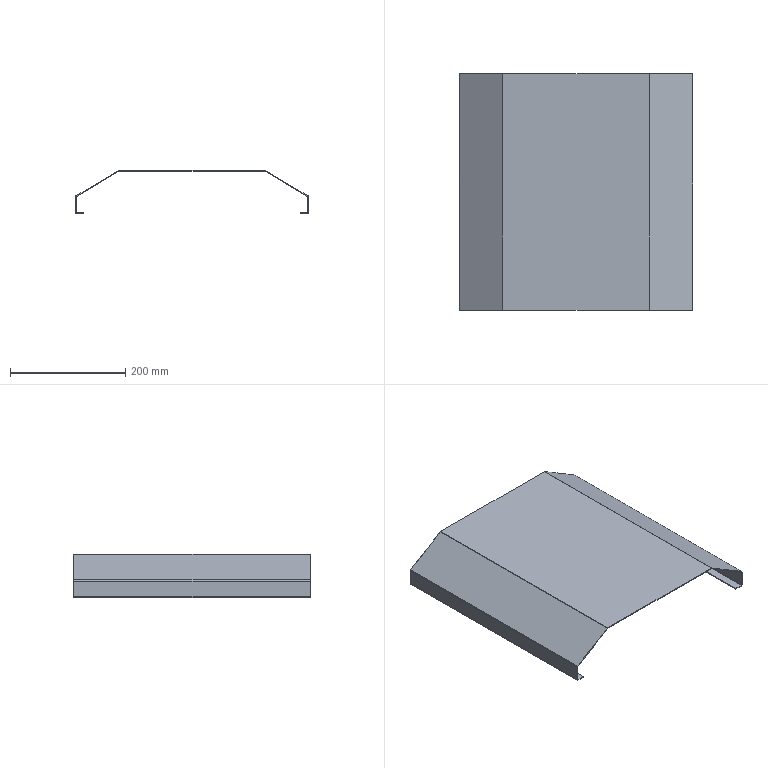Part | SolidWorks | features BaseBody 1 | 1 solid | 38 faces | box 405 x 410 x 75 mm | volume 315141 mm3 | cylinder 20 | plane 18 | commonest cylinder face diameters 6.8 x8 1.473 x6 4.473 x6
STEP:
#1=CARTESIAN_POINT('',(201.,65.5,-54.6));
#2=VERTEX_POINT('',#1);
#3=CARTESIAN_POINT('',(201.,65.5,-61.4));
#4=VERTEX_POINT('',#3);
#5=CARTESIAN_POINT('',(201.,65.5,-58.));
#6=DIRECTION('',(1.,0.,0.));
#7=DIRECTION('',(0.,0.,-1.));
#8=AXIS2_PLACEMENT_3D('',#5,#6,#7);
#9=CIRCLE('',#8,3.4);
#10=EDGE_CURVE('',#2,#4,#9,.T.);
#11=ORIENTED_EDGE('',*,*,#10,.F.);
#12=CARTESIAN_POINT('',(202.5,65.5,-54.6));
#13=VERTEX_POINT('',#12);
#14=CARTESIAN_POINT('',(202.5,65.5,-54.6));
#15=DIRECTION('',(1.,0.,0.));
#16=VECTOR('',#15,1000.);
#17=LINE('',#14,#16);
#18=EDGE_CURVE('',#2,#13,#17,.T.);
#19=ORIENTED_EDGE('',*,*,#18,.T.);
#20=CARTESIAN_POINT('',(202.5,65.5,-61.4));
#21=VERTEX_POINT('',#20);
#22=CARTESIAN_POINT('',(202.5,65.5,-58.));
#23=DIRECTION('',(-1.,0.,0.));
#24=DIRECTION('',(0.,0.,-1.));
#25=AXIS2_PLACEMENT_3D('',#22,#23,#24);
#26=CIRCLE('',#25,3.4);
#27=EDGE_CURVE('',#21,#13,#26,.T.);
#28=ORIENTED_EDGE('',*,*,#27,.F.);
#29=CARTESIAN_POINT('',(202.5,65.5,-61.4));
#30=DIRECTION('',(1.,0.,0.));
#31=VECTOR('',#30,1000.);
#32=LINE('',#29,#31);
#33=EDGE_CURVE('',#4,#21,#32,.T.);
#34=ORIENTED_EDGE('',*,*,#33,.F.);
#35=EDGE_LOOP('',(#11,#19,#28,#34));
#36=FACE_OUTER_BOUND('',#35,.T.);
#37=CARTESIAN_POINT('',(202.5,65.5,-58.));
#38=DIRECTION('',(1.,0.,0.));
#39=DIRECTION('',(0.,0.,-1.));
#40=AXIS2_PLACEMENT_3D('',#37,#38,#39);
#41=CYLINDRICAL_SURFACE('',#40,3.4);
#42=ADVANCED_FACE('',(#36),#41,.F.);
#43=CARTESIAN_POINT('',(201.,101.5,-54.6));
#44=VERTEX_POINT('',#43);
#45=CARTESIAN_POINT('',(201.,101.5,-61.4));
#46=VERTEX_POINT('',#45);
#47=CARTESIAN_POINT('',(201.,101.5,-58.));
#48=DIRECTION('',(1.,0.,0.));
#49=DIRECTION('',(0.,0.,-1.));
#50=AXIS2_PLACEMENT_3D('',#47,#48,#49);
#51=CIRCLE('',#50,3.4);
#52=EDGE_CURVE('',#44,#46,#51,.T.);
#53=ORIENTED_EDGE('',*,*,#52,.F.);
#54=CARTESIAN_POINT('',(202.5,101.5,-54.6));
#55=VERTEX_POINT('',#54);
#56=CARTESIAN_POINT('',(202.5,101.5,-54.6));
#57=DIRECTION('',(1.,0.,0.));
#58=VECTOR('',#57,1000.);
#59=LINE('',#56,#58);
#60=EDGE_CURVE('',#44,#55,#59,.T.);
#61=ORIENTED_EDGE('',*,*,#60,.T.);
#62=CARTESIAN_POINT('',(202.5,101.5,-61.4));
#63=VERTEX_POINT('',#62);
#64=CARTESIAN_POINT('',(202.5,101.5,-58.));
#65=DIRECTION('',(-1.,0.,0.));
#66=DIRECTION('',(0.,0.,-1.));
#67=AXIS2_PLACEMENT_3D('',#64,#65,#66);
#68=CIRCLE('',#67,3.4);
#69=EDGE_CURVE('',#63,#55,#68,.T.);
#70=ORIENTED_EDGE('',*,*,#69,.F.);
#71=CARTESIAN_POINT('',(202.5,101.5,-61.4));
#72=DIRECTION('',(1.,0.,0.));
#73=VECTOR('',#72,1000.);
#74=LINE('',#71,#73);
#75=EDGE_CURVE('',#46,#63,#74,.T.);
#76=ORIENTED_EDGE('',*,*,#75,.F.);
#77=EDGE_LOOP('',(#53,#61,#70,#76));
#78=FACE_OUTER_BOUND('',#77,.T.);
#79=CARTESIAN_POINT('',(202.5,101.5,-58.));
#80=DIRECTION('',(1.,0.,0.));
#81=DIRECTION('',(0.,0.,-1.));
#82=AXIS2_PLACEMENT_3D('',#79,#80,#81);
#83=CYLINDRICAL_SURFACE('',#82,3.4);
#84=ADVANCED_FACE('',(#78),#83,.F.);
#85=CARTESIAN_POINT('',(201.,241.5,-54.6));
#86=VERTEX_POINT('',#85);
#87=CARTESIAN_POINT('',(201.,241.5,-61.4));
#88=VERTEX_POINT('',#87);
#89=CARTESIAN_POINT('',(201.,241.5,-58.));
#90=DIRECTION('',(1.,0.,0.));
#91=DIRECTION('',(0.,0.,-1.));
#92=AXIS2_PLACEMENT_3D('',#89,#90,#91);
#93=CIRCLE('',#92,3.4);
#94=EDGE_CURVE('',#86,#88,#93,.T.);
#95=ORIENTED_EDGE('',*,*,#94,.F.);
#96=CARTESIAN_POINT('',(202.5,241.5,-54.6));
#97=VERTEX_POINT('',#96);
#98=CARTESIAN_POINT('',(202.5,241.5,-54.6));
#99=DIRECTION('',(1.,0.,0.));
#100=VECTOR('',#99,1000.);
#101=LINE('',#98,#100);
#102=EDGE_CURVE('',#86,#97,#101,.T.);
#103=ORIENTED_EDGE('',*,*,#102,.T.);
#104=CARTESIAN_POINT('',(202.5,241.5,-61.4));
#105=VERTEX_POINT('',#104);
#106=CARTESIAN_POINT('',(202.5,241.5,-58.));
#107=DIRECTION('',(-1.,0.,0.));
#108=DIRECTION('',(0.,0.,-1.));
#109=AXIS2_PLACEMENT_3D('',#106,#107,#108);
#110=CIRCLE('',#109,3.4);
#111=EDGE_CURVE('',#105,#97,#110,.T.);
#112=ORIENTED_EDGE('',*,*,#111,.F.);
#113=CARTESIAN_POINT('',(202.5,241.5,-61.4));
#114=DIRECTION('',(1.,0.,0.));
#115=VECTOR('',#114,1000.);
#116=LINE('',#113,#115);
#117=EDGE_CURVE('',#88,#105,#116,.T.);
#118=ORIENTED_EDGE('',*,*,#117,.F.);
#119=EDGE_LOOP('',(#95,#103,#112,#118));
#120=FACE_OUTER_BOUND('',#119,.T.);
#121=CARTESIAN_POINT('',(202.5,241.5,-58.));
#122=DIRECTION('',(1.,0.,0.));
#123=DIRECTION('',(0.,0.,-1.));
#124=AXIS2_PLACEMENT_3D('',#121,#122,#123);
#125=CYLINDRICAL_SURFACE('',#124,3.4);
#126=ADVANCED_FACE('',(#120),#125,.F.);
#127=CARTESIAN_POINT('',(201.,277.5,-54.6));
#128=VERTEX_POINT('',#127);
#129=CARTESIAN_POINT('',(201.,277.5,-61.4));
#130=VERTEX_POINT('',#129);
#131=CARTESIAN_POINT('',(201.,277.5,-58.));
#132=DIRECTION('',(1.,0.,0.));
#133=DIRECTION('',(0.,0.,-1.));
#134=AXIS2_PLACEMENT_3D('',#131,#132,#133);
#135=CIRCLE('',#134,3.4);
#136=EDGE_CURVE('',#128,#130,#135,.T.);
#137=ORIENTED_EDGE('',*,*,#136,.F.);
#138=CARTESIAN_POINT('',(202.5,277.5,-54.6));
#139=VERTEX_POINT('',#138);
#140=CARTESIAN_POINT('',(202.5,277.5,-54.6));
#141=DIRECTION('',(1.,0.,0.));
#142=VECTOR('',#141,1000.);
#143=LINE('',#140,#142);
#144=EDGE_CURVE('',#128,#139,#143,.T.);
#145=ORIENTED_EDGE('',*,*,#144,.T.);
#146=CARTESIAN_POINT('',(202.5,277.5,-61.4));
#147=VERTEX_POINT('',#146);
#148=CARTESIAN_POINT('',(202.5,277.5,-58.));
#149=DIRECTION('',(-1.,0.,0.));
#150=DIRECTION('',(0.,0.,-1.));
#151=AXIS2_PLACEMENT_3D('',#148,#149,#150);
#152=CIRCLE('',#151,3.4);
#153=EDGE_CURVE('',#147,#139,#152,.T.);
#154=ORIENTED_EDGE('',*,*,#153,.F.);
#155=CARTESIAN_POINT('',(202.5,277.5,-61.4));
#156=DIRECTION('',(1.,0.,0.));
#157=VECTOR('',#156,1000.);
#158=LINE('',#155,#157);
#159=EDGE_CURVE('',#130,#147,#158,.T.);
#160=ORIENTED_EDGE('',*,*,#159,.F.);
#161=EDGE_LOOP('',(#137,#145,#154,#160));
#162=FACE_OUTER_BOUND('',#161,.T.);
#163=CARTESIAN_POINT('',(202.5,277.5,-58.));
#164=DIRECTION('',(1.,0.,0.));
#165=DIRECTION('',(0.,0.,-1.));
#166=AXIS2_PLACEMENT_3D('',#163,#164,#165);
#167=CYLINDRICAL_SURFACE('',#166,3.4);
#168=ADVANCED_FACE('',(#162),#167,.F.);
#169=CARTESIAN_POINT('',(-126.88,410.,-1.5));
#170=VERTEX_POINT('',#169);
#171=CARTESIAN_POINT('',(126.88,410.,-1.5));
#172=VERTEX_POINT('',#171);
#173=CARTESIAN_POINT('',(-127.5,410.,-1.5));
#174=DIRECTION('',(1.,0.,0.));
#175=VECTOR('',#174,1000.);
#176=LINE('',#173,#175);
#177=EDGE_CURVE('',#170,#172,#176,.T.);
#178=ORIENTED_EDGE('',*,*,#177,.T.);
#179=CARTESIAN_POINT('',(126.88,0.,-1.5));
#180=VERTEX_POINT('',#179);
#181=CARTESIAN_POINT('',(126.88,410.,-1.5));
#182=DIRECTION('',(0.,-1.,0.));
#183=VECTOR('',#182,1000.);
#184=LINE('',#181,#183);
#185=EDGE_CURVE('',#172,#180,#184,.T.);
#186=ORIENTED_EDGE('',*,*,#185,.T.);
#187=CARTESIAN_POINT('',(-126.88,0.,-1.5));
#188=VERTEX_POINT('',#187);
#189=CARTESIAN_POINT('',(-127.5,0.,-1.5));
#190=DIRECTION('',(-1.,0.,0.));
#191=VECTOR('',#190,1000.);
#192=LINE('',#189,#191);
#193=EDGE_CURVE('',#180,#188,#192,.T.);
#194=ORIENTED_EDGE('',*,*,#193,.T.);
#195=CARTESIAN_POINT('',(-126.88,410.,-1.5));
#196=DIRECTION('',(0.,1.,0.));
#197=VECTOR('',#196,1000.);
#198=LINE('',#195,#197);
#199=EDGE_CURVE('',#188,#170,#198,.T.);
#200=ORIENTED_EDGE('',*,*,#199,.T.);
#201=EDGE_LOOP('',(#178,#186,#194,#200));
#202=FACE_OUTER_BOUND('',#201,.T.);
#203=CARTESIAN_POINT('',(-127.5,410.,-1.5));
#204=DIRECTION('',(0.,0.,-1.));
#205=DIRECTION('',(-1.,0.,0.));
#206=AXIS2_PLACEMENT_3D('',#203,#204,#205);
#207=PLANE('',#206);
#208=ADVANCED_FACE('',(#202),#207,.T.);
#209=ORIENTED_EDGE('',*,*,#185,.F.);
#210=CARTESIAN_POINT('',(127.259,410.,-1.605));
#211=VERTEX_POINT('',#210);
#212=CARTESIAN_POINT('',(126.88,410.,-2.237));
#213=DIRECTION('',(0.,-1.,0.));
#214=DIRECTION('',(0.,0.,-1.));
#215=AXIS2_PLACEMENT_3D('',#212,#213,#214);
#216=CIRCLE('',#215,0.7366);
#217=EDGE_CURVE('',#211,#172,#216,.T.);
#218=ORIENTED_EDGE('',*,*,#217,.F.);
#219=CARTESIAN_POINT('',(127.259,0.,-1.605));
#220=VERTEX_POINT('',#219);
#221=CARTESIAN_POINT('',(127.259,410.,-1.605));
#222=DIRECTION('',(0.,1.,0.));
#223=VECTOR('',#222,1000.);
#224=LINE('',#221,#223);
#225=EDGE_CURVE('',#220,#211,#224,.T.);
#226=ORIENTED_EDGE('',*,*,#225,.F.);
#227=CARTESIAN_POINT('',(126.88,0.,-2.237));
#228=DIRECTION('',(0.,1.,0.));
#229=DIRECTION('',(0.,0.,-1.));
#230=AXIS2_PLACEMENT_3D('',#227,#228,#229);
#231=CIRCLE('',#230,0.7366);
#232=EDGE_CURVE('',#180,#220,#231,.T.);
#233=ORIENTED_EDGE('',*,*,#232,.F.);
#234=EDGE_LOOP('',(#209,#218,#226,#233));
#235=FACE_OUTER_BOUND('',#234,.T.);
#236=CARTESIAN_POINT('',(126.88,410.,-2.237));
#237=DIRECTION('',(0.,-1.,0.));
#238=DIRECTION('',(0.,0.,-1.));
#239=AXIS2_PLACEMENT_3D('',#236,#237,#238);
#240=CYLINDRICAL_SURFACE('',#239,0.7366);
#241=ADVANCED_FACE('',(#235),#240,.F.);
#242=ORIENTED_EDGE('',*,*,#177,.F.);
#243=CARTESIAN_POINT('',(-127.259,410.,-1.605));
#244=VERTEX_POINT('',#243);
#245=CARTESIAN_POINT('',(-126.88,410.,-2.237));
#246=DIRECTION('',(0.,-1.,0.));
#247=DIRECTION('',(0.,0.,-1.));
#248=AXIS2_PLACEMENT_3D('',#245,#246,#247);
#249=CIRCLE('',#248,0.7366);
#250=EDGE_CURVE('',#170,#244,#249,.T.);
#251=ORIENTED_EDGE('',*,*,#250,.T.);
#252=CARTESIAN_POINT('',(-200.642,410.,-45.635));
#253=VERTEX_POINT('',#252);
#254=CARTESIAN_POINT('',(-126.728,410.,-1.286));
#255=DIRECTION('',(0.8575,0.,0.5145));
#256=VECTOR('',#255,1000.);
#257=LINE('',#254,#256);
#258=EDGE_CURVE('',#253,#244,#257,.T.);
#259=ORIENTED_EDGE('',*,*,#258,.F.);
#260=CARTESIAN_POINT('',(-201.,410.,-46.266));
#261=VERTEX_POINT('',#260);
#262=CARTESIAN_POINT('',(-200.263,410.,-46.266));
#263=DIRECTION('',(0.,-1.,0.));
#264=DIRECTION('',(0.,0.,-1.));
#265=AXIS2_PLACEMENT_3D('',#262,#263,#264);
#266=CIRCLE('',#265,0.7366);
#267=EDGE_CURVE('',#253,#261,#266,.T.);
#268=ORIENTED_EDGE('',*,*,#267,.T.);
#269=CARTESIAN_POINT('',(-201.,410.,-72.763));
#270=VERTEX_POINT('',#269);
#271=CARTESIAN_POINT('',(-201.,410.,-45.));
#272=DIRECTION('',(0.,0.,1.));
#273=VECTOR('',#272,1000.);
#274=LINE('',#271,#273);
#275=EDGE_CURVE('',#270,#261,#274,.T.);
#276=ORIENTED_EDGE('',*,*,#275,.F.);
#277=CARTESIAN_POINT('',(-200.263,410.,-73.5));
#278=VERTEX_POINT('',#277);
#279=CARTESIAN_POINT('',(-200.263,410.,-72.763));
#280=DIRECTION('',(0.,-1.,0.));
#281=DIRECTION('',(0.,0.,-1.));
#282=AXIS2_PLACEMENT_3D('',#279,#280,#281);
#283=CIRCLE('',#282,0.7366);
#284=EDGE_CURVE('',#270,#278,#283,.T.);
#285=ORIENTED_EDGE('',*,*,#284,.T.);
#286=CARTESIAN_POINT('',(-187.5,410.,-73.5));
#287=VERTEX_POINT('',#286);
#288=CARTESIAN_POINT('',(-202.5,410.,-73.5));
#289=DIRECTION('',(-1.,0.,0.));
#290=VECTOR('',#289,1000.);
#291=LINE('',#288,#290);
#292=EDGE_CURVE('',#287,#278,#291,.T.);
#293=ORIENTED_EDGE('',*,*,#292,.F.);
#294=CARTESIAN_POINT('',(-187.5,410.,-75.));
#295=VERTEX_POINT('',#294);
#296=CARTESIAN_POINT('',(-187.5,410.,-72.763));
#297=DIRECTION('',(0.,0.,-1.));
#298=VECTOR('',#297,1000.);
#299=LINE('',#296,#298);
#300=EDGE_CURVE('',#287,#295,#299,.T.);
#301=ORIENTED_EDGE('',*,*,#300,.T.);
#302=CARTESIAN_POINT('',(-200.263,410.,-75.));
#303=VERTEX_POINT('',#302);
#304=CARTESIAN_POINT('',(-201.,410.,-75.));
#305=DIRECTION('',(-1.,0.,0.));
#306=VECTOR('',#305,1000.);
#307=LINE('',#304,#306);
#308=EDGE_CURVE('',#295,#303,#307,.T.);
#309=ORIENTED_EDGE('',*,*,#308,.T.);
#310=CARTESIAN_POINT('',(-202.5,410.,-72.763));
#311=VERTEX_POINT('',#310);
#312=CARTESIAN_POINT('',(-200.263,410.,-72.763));
#313=DIRECTION('',(0.,-1.,0.));
#314=DIRECTION('',(0.,0.,-1.));
#315=AXIS2_PLACEMENT_3D('',#312,#313,#314);
#316=CIRCLE('',#315,2.237);
#317=EDGE_CURVE('',#311,#303,#316,.T.);
#318=ORIENTED_EDGE('',*,*,#317,.F.);
#319=CARTESIAN_POINT('',(-202.5,410.,-46.266));
#320=VERTEX_POINT('',#319);
#321=CARTESIAN_POINT('',(-202.5,410.,-45.635));
#322=DIRECTION('',(0.,0.,1.));
#323=VECTOR('',#322,1000.);
#324=LINE('',#321,#323);
#325=EDGE_CURVE('',#311,#320,#324,.T.);
#326=ORIENTED_EDGE('',*,*,#325,.T.);
#327=CARTESIAN_POINT('',(-201.414,410.,-44.348));
#328=VERTEX_POINT('',#327);
#329=CARTESIAN_POINT('',(-200.263,410.,-46.266));
#330=DIRECTION('',(0.,-1.,0.));
#331=DIRECTION('',(0.,0.,-1.));
#332=AXIS2_PLACEMENT_3D('',#329,#330,#331);
#333=CIRCLE('',#332,2.237);
#334=EDGE_CURVE('',#328,#320,#333,.T.);
#335=ORIENTED_EDGE('',*,*,#334,.F.);
#336=CARTESIAN_POINT('',(-128.031,410.,-0.3187));
#337=VERTEX_POINT('',#336);
#338=CARTESIAN_POINT('',(-201.414,410.,-44.348));
#339=DIRECTION('',(0.8575,0.,0.5145));
#340=VECTOR('',#339,1000.);
#341=LINE('',#338,#340);
#342=EDGE_CURVE('',#328,#337,#341,.T.);
#343=ORIENTED_EDGE('',*,*,#342,.T.);
#344=CARTESIAN_POINT('',(-126.88,410.,0.));
#345=VERTEX_POINT('',#344);
#346=CARTESIAN_POINT('',(-126.88,410.,-2.237));
#347=DIRECTION('',(0.,-1.,0.));
#348=DIRECTION('',(0.,0.,-1.));
#349=AXIS2_PLACEMENT_3D('',#346,#347,#348);
#350=CIRCLE('',#349,2.237);
#351=EDGE_CURVE('',#345,#337,#350,.T.);
#352=ORIENTED_EDGE('',*,*,#351,.F.);
#353=CARTESIAN_POINT('',(126.88,410.,0.));
#354=VERTEX_POINT('',#353);
#355=CARTESIAN_POINT('',(127.259,410.,0.));
#356=DIRECTION('',(1.,0.,0.));
#357=VECTOR('',#356,1000.);
#358=LINE('',#355,#357);
#359=EDGE_CURVE('',#345,#354,#358,.T.);
#360=ORIENTED_EDGE('',*,*,#359,.T.);
#361=CARTESIAN_POINT('',(128.031,410.,-0.3187));
#362=VERTEX_POINT('',#361);
#363=CARTESIAN_POINT('',(126.88,410.,-2.237));
#364=DIRECTION('',(0.,-1.,0.));
#365=DIRECTION('',(0.,0.,-1.));
#366=AXIS2_PLACEMENT_3D('',#363,#364,#365);
#367=CIRCLE('',#366,2.237);
#368=EDGE_CURVE('',#362,#354,#367,.T.);
#369=ORIENTED_EDGE('',*,*,#368,.F.);
#370=CARTESIAN_POINT('',(201.414,410.,-44.348));
#371=VERTEX_POINT('',#370);
#372=CARTESIAN_POINT('',(128.031,410.,-0.3187));
#373=DIRECTION('',(0.8575,0.,-0.5145));
#374=VECTOR('',#373,1000.);
#375=LINE('',#372,#374);
#376=EDGE_CURVE('',#362,#371,#375,.T.);
#377=ORIENTED_EDGE('',*,*,#376,.T.);
#378=CARTESIAN_POINT('',(202.5,410.,-46.266));
#379=VERTEX_POINT('',#378);
#380=CARTESIAN_POINT('',(200.263,410.,-46.266));
#381=DIRECTION('',(0.,-1.,0.));
#382=DIRECTION('',(0.,0.,-1.));
#383=AXIS2_PLACEMENT_3D('',#380,#381,#382);
#384=CIRCLE('',#383,2.237);
#385=EDGE_CURVE('',#379,#371,#384,.T.);
#386=ORIENTED_EDGE('',*,*,#385,.F.);
#387=CARTESIAN_POINT('',(202.5,410.,-72.763));
#388=VERTEX_POINT('',#387);
#389=CARTESIAN_POINT('',(202.5,410.,-73.5));
#390=DIRECTION('',(0.,0.,-1.));
#391=VECTOR('',#390,1000.);
#392=LINE('',#389,#391);
#393=EDGE_CURVE('',#379,#388,#392,.T.);
#394=ORIENTED_EDGE('',*,*,#393,.T.);
#395=CARTESIAN_POINT('',(200.263,410.,-75.));
#396=VERTEX_POINT('',#395);
#397=CARTESIAN_POINT('',(200.263,410.,-72.763));
#398=DIRECTION('',(0.,-1.,0.));
#399=DIRECTION('',(0.,0.,-1.));
#400=AXIS2_PLACEMENT_3D('',#397,#398,#399);
#401=CIRCLE('',#400,2.237);
#402=EDGE_CURVE('',#396,#388,#401,.T.);
#403=ORIENTED_EDGE('',*,*,#402,.F.);
#404=CARTESIAN_POINT('',(187.5,410.,-75.));
#405=VERTEX_POINT('',#404);
#406=CARTESIAN_POINT('',(200.263,410.,-75.));
#407=DIRECTION('',(-1.,0.,0.));
#408=VECTOR('',#407,1000.);
#409=LINE('',#406,#408);
#410=EDGE_CURVE('',#396,#405,#409,.T.);
#411=ORIENTED_EDGE('',*,*,#410,.T.);
#412=CARTESIAN_POINT('',(187.5,410.,-73.5));
#413=VERTEX_POINT('',#412);
#414=CARTESIAN_POINT('',(187.5,410.,-73.5));
#415=DIRECTION('',(0.,0.,-1.));
#416=VECTOR('',#415,1000.);
#417=LINE('',#414,#416);
#418=EDGE_CURVE('',#413,#405,#417,.T.);
#419=ORIENTED_EDGE('',*,*,#418,.F.);
#420=CARTESIAN_POINT('',(200.263,410.,-73.5));
#421=VERTEX_POINT('',#420);
#422=CARTESIAN_POINT('',(202.5,410.,-73.5));
#423=DIRECTION('',(-1.,0.,0.));
#424=VECTOR('',#423,1000.);
#425=LINE('',#422,#424);
#426=EDGE_CURVE('',#421,#413,#425,.T.);
#427=ORIENTED_EDGE('',*,*,#426,.F.);
#428=CARTESIAN_POINT('',(201.,410.,-72.763));
#429=VERTEX_POINT('',#428);
#430=CARTESIAN_POINT('',(200.263,410.,-72.763));
#431=DIRECTION('',(0.,-1.,0.));
#432=DIRECTION('',(0.,0.,-1.));
#433=AXIS2_PLACEMENT_3D('',#430,#431,#432);
#434=CIRCLE('',#433,0.7366);
#435=EDGE_CURVE('',#421,#429,#434,.T.);
#436=ORIENTED_EDGE('',*,*,#435,.T.);
#437=CARTESIAN_POINT('',(201.,410.,-46.266));
#438=VERTEX_POINT('',#437);
#439=CARTESIAN_POINT('',(201.,410.,-45.));
#440=DIRECTION('',(0.,0.,-1.));
#441=VECTOR('',#440,1000.);
#442=LINE('',#439,#441);
#443=EDGE_CURVE('',#438,#429,#442,.T.);
#444=ORIENTED_EDGE('',*,*,#443,.F.);
#445=CARTESIAN_POINT('',(200.642,410.,-45.635));
#446=VERTEX_POINT('',#445);
#447=CARTESIAN_POINT('',(200.263,410.,-46.266));
#448=DIRECTION('',(0.,-1.,0.));
#449=DIRECTION('',(0.,0.,-1.));
#450=AXIS2_PLACEMENT_3D('',#447,#448,#449);
#451=CIRCLE('',#450,0.7366);
#452=EDGE_CURVE('',#438,#446,#451,.T.);
#453=ORIENTED_EDGE('',*,*,#452,.T.);
#454=CARTESIAN_POINT('',(126.728,410.,-1.286));
#455=DIRECTION('',(0.8575,0.,-0.5145));
#456=VECTOR('',#455,1000.);
#457=LINE('',#454,#456);
#458=EDGE_CURVE('',#211,#446,#457,.T.);
#459=ORIENTED_EDGE('',*,*,#458,.F.);
#460=ORIENTED_EDGE('',*,*,#217,.T.);
#461=EDGE_LOOP('',(#242,#251,#259,#268,#276,#285,#293,#301,#309,#318,#326,#335,#343,#352,#360,#369,#377,#386,#394,#403,#411,#419,#427,#436,#444,#453,#459,#460));
#462=FACE_OUTER_BOUND('',#461,.T.);
#463=CARTESIAN_POINT('',(127.259,410.,-1.605));
#464=DIRECTION('',(0.,1.,0.));
#465=DIRECTION('',(0.,0.,1.));
#466=AXIS2_PLACEMENT_3D('',#463,#464,#465);
#467=PLANE('',#466);
#468=ADVANCED_FACE('',(#462),#467,.T.);
#469=CARTESIAN_POINT('',(-127.259,0.,-1.605));
#470=VERTEX_POINT('',#469);
#471=CARTESIAN_POINT('',(-127.259,410.,-1.605));
#472=DIRECTION('',(0.,-1.,0.));
#473=VECTOR('',#472,1000.);
#474=LINE('',#471,#473);
#475=EDGE_CURVE('',#244,#470,#474,.T.);
#476=ORIENTED_EDGE('',*,*,#475,.F.);
#477=ORIENTED_EDGE('',*,*,#250,.F.);
#478=ORIENTED_EDGE('',*,*,#199,.F.);
#479=CARTESIAN_POINT('',(-126.88,0.,-2.237));
#480=DIRECTION('',(0.,1.,0.));
#481=DIRECTION('',(0.,0.,-1.));
#482=AXIS2_PLACEMENT_3D('',#479,#480,#481);
#483=CIRCLE('',#482,0.7366);
#484=EDGE_CURVE('',#470,#188,#483,.T.);
#485=ORIENTED_EDGE('',*,*,#484,.F.);
#486=EDGE_LOOP('',(#476,#477,#478,#485));
#487=FACE_OUTER_BOUND('',#486,.T.);
#488=CARTESIAN_POINT('',(-126.88,410.,-2.237));
#489=DIRECTION('',(0.,-1.,0.));
#490=DIRECTION('',(0.,0.,-1.));
#491=AXIS2_PLACEMENT_3D('',#488,#489,#490);
#492=CYLINDRICAL_SURFACE('',#491,0.7366);
#493=ADVANCED_FACE('',(#487),#492,.F.);
#494=ORIENTED_EDGE('',*,*,#193,.F.);
#495=ORIENTED_EDGE('',*,*,#232,.T.);
#496=CARTESIAN_POINT('',(200.642,0.,-45.635));
#497=VERTEX_POINT('',#496);
#498=CARTESIAN_POINT('',(126.728,0.,-1.286));
#499=DIRECTION('',(-0.8575,0.,0.5145));
#500=VECTOR('',#499,1000.);
#501=LINE('',#498,#500);
#502=EDGE_CURVE('',#497,#220,#501,.T.);
#503=ORIENTED_EDGE('',*,*,#502,.F.);
#504=CARTESIAN_POINT('',(201.,0.,-46.266));
#505=VERTEX_POINT('',#504);
#506=CARTESIAN_POINT('',(200.263,0.,-46.266));
#507=DIRECTION('',(0.,1.,0.));
#508=DIRECTION('',(0.,0.,-1.));
#509=AXIS2_PLACEMENT_3D('',#506,#507,#508);
#510=CIRCLE('',#509,0.7366);
#511=EDGE_CURVE('',#497,#505,#510,.T.);
#512=ORIENTED_EDGE('',*,*,#511,.T.);
#513=CARTESIAN_POINT('',(201.,0.,-72.763));
#514=VERTEX_POINT('',#513);
#515=CARTESIAN_POINT('',(201.,0.,-45.));
#516=DIRECTION('',(0.,0.,1.));
#517=VECTOR('',#516,1000.);
#518=LINE('',#515,#517);
#519=EDGE_CURVE('',#514,#505,#518,.T.);
#520=ORIENTED_EDGE('',*,*,#519,.F.);
#521=CARTESIAN_POINT('',(200.263,0.,-73.5));
#522=VERTEX_POINT('',#521);
#523=CARTESIAN_POINT('',(200.263,0.,-72.763));
#524=DIRECTION('',(0.,1.,0.));
#525=DIRECTION('',(0.,0.,-1.));
#526=AXIS2_PLACEMENT_3D('',#523,#524,#525);
#527=CIRCLE('',#526,0.7366);
#528=EDGE_CURVE('',#514,#522,#527,.T.);
#529=ORIENTED_EDGE('',*,*,#528,.T.);
#530=CARTESIAN_POINT('',(187.5,0.,-73.5));
#531=VERTEX_POINT('',#530);
#532=CARTESIAN_POINT('',(202.5,0.,-73.5));
#533=DIRECTION('',(1.,0.,0.));
#534=VECTOR('',#533,1000.);
#535=LINE('',#532,#534);
#536=EDGE_CURVE('',#531,#522,#535,.T.);
#537=ORIENTED_EDGE('',*,*,#536,.F.);
#538=CARTESIAN_POINT('',(187.5,0.,-75.));
#539=VERTEX_POINT('',#538);
#540=CARTESIAN_POINT('',(187.5,0.,-73.5));
#541=DIRECTION('',(0.,0.,1.));
#542=VECTOR('',#541,1000.);
#543=LINE('',#540,#542);
#544=EDGE_CURVE('',#539,#531,#543,.T.);
#545=ORIENTED_EDGE('',*,*,#544,.F.);
#546=CARTESIAN_POINT('',(200.263,0.,-75.));
#547=VERTEX_POINT('',#546);
#548=CARTESIAN_POINT('',(201.,0.,-75.));
#549=DIRECTION('',(1.,0.,0.));
#550=VECTOR('',#549,1000.);
#551=LINE('',#548,#550);
#552=EDGE_CURVE('',#539,#547,#551,.T.);
#553=ORIENTED_EDGE('',*,*,#552,.T.);
#554=CARTESIAN_POINT('',(202.5,0.,-72.763));
#555=VERTEX_POINT('',#554);
#556=CARTESIAN_POINT('',(200.263,0.,-72.763));
#557=DIRECTION('',(0.,1.,0.));
#558=DIRECTION('',(0.,0.,-1.));
#559=AXIS2_PLACEMENT_3D('',#556,#557,#558);
#560=CIRCLE('',#559,2.237);
#561=EDGE_CURVE('',#555,#547,#560,.T.);
#562=ORIENTED_EDGE('',*,*,#561,.F.);
#563=CARTESIAN_POINT('',(202.5,0.,-46.266));
#564=VERTEX_POINT('',#563);
#565=CARTESIAN_POINT('',(202.5,0.,-45.635));
#566=DIRECTION('',(0.,0.,1.));
#567=VECTOR('',#566,1000.);
#568=LINE('',#565,#567);
#569=EDGE_CURVE('',#555,#564,#568,.T.);
#570=ORIENTED_EDGE('',*,*,#569,.T.);
#571=CARTESIAN_POINT('',(201.414,0.,-44.348));
#572=VERTEX_POINT('',#571);
#573=CARTESIAN_POINT('',(200.263,0.,-46.266));
#574=DIRECTION('',(0.,1.,0.));
#575=DIRECTION('',(0.,0.,-1.));
#576=AXIS2_PLACEMENT_3D('',#573,#574,#575);
#577=CIRCLE('',#576,2.237);
#578=EDGE_CURVE('',#572,#564,#577,.T.);
#579=ORIENTED_EDGE('',*,*,#578,.F.);
#580=CARTESIAN_POINT('',(128.031,0.,-0.3187));
#581=VERTEX_POINT('',#580);
#582=CARTESIAN_POINT('',(201.414,0.,-44.348));
#583=DIRECTION('',(-0.8575,0.,0.5145));
#584=VECTOR('',#583,1000.);
#585=LINE('',#582,#584);
#586=EDGE_CURVE('',#572,#581,#585,.T.);
#587=ORIENTED_EDGE('',*,*,#586,.T.);
#588=CARTESIAN_POINT('',(126.88,0.,0.));
#589=VERTEX_POINT('',#588);
#590=CARTESIAN_POINT('',(126.88,0.,-2.237));
#591=DIRECTION('',(0.,-1.,0.));
#592=DIRECTION('',(0.,0.,-1.));
#593=AXIS2_PLACEMENT_3D('',#590,#591,#592);
#594=CIRCLE('',#593,2.237);
#595=EDGE_CURVE('',#581,#589,#594,.T.);
#596=ORIENTED_EDGE('',*,*,#595,.T.);
#597=CARTESIAN_POINT('',(-126.88,0.,0.));
#598=VERTEX_POINT('',#597);
#599=CARTESIAN_POINT('',(-127.259,0.,0.));
#600=DIRECTION('',(-1.,0.,0.));
#601=VECTOR('',#600,1000.);
#602=LINE('',#599,#601);
#603=EDGE_CURVE('',#589,#598,#602,.T.);
#604=ORIENTED_EDGE('',*,*,#603,.T.);
#605=CARTESIAN_POINT('',(-128.031,0.,-0.3187));
#606=VERTEX_POINT('',#605);
#607=CARTESIAN_POINT('',(-126.88,0.,-2.237));
#608=DIRECTION('',(0.,-1.,0.));
#609=DIRECTION('',(0.,0.,-1.));
#610=AXIS2_PLACEMENT_3D('',#607,#608,#609);
#611=CIRCLE('',#610,2.237);
#612=EDGE_CURVE('',#598,#606,#611,.T.);
#613=ORIENTED_EDGE('',*,*,#612,.T.);
#614=CARTESIAN_POINT('',(-201.414,0.,-44.348));
#615=VERTEX_POINT('',#614);
#616=CARTESIAN_POINT('',(-128.031,0.,-0.3187));
#617=DIRECTION('',(-0.8575,0.,-0.5145));
#618=VECTOR('',#617,1000.);
#619=LINE('',#616,#618);
#620=EDGE_CURVE('',#606,#615,#619,.T.);
#621=ORIENTED_EDGE('',*,*,#620,.T.);
#622=CARTESIAN_POINT('',(-202.5,0.,-46.266));
#623=VERTEX_POINT('',#622);
#624=CARTESIAN_POINT('',(-200.263,0.,-46.266));
#625=DIRECTION('',(0.,1.,0.));
#626=DIRECTION('',(0.,0.,-1.));
#627=AXIS2_PLACEMENT_3D('',#624,#625,#626);
#628=CIRCLE('',#627,2.237);
#629=EDGE_CURVE('',#623,#615,#628,.T.);
#630=ORIENTED_EDGE('',*,*,#629,.F.);
#631=CARTESIAN_POINT('',(-202.5,0.,-72.763));
#632=VERTEX_POINT('',#631);
#633=CARTESIAN_POINT('',(-202.5,0.,-73.5));
#634=DIRECTION('',(0.,0.,-1.));
#635=VECTOR('',#634,1000.);
#636=LINE('',#633,#635);
#637=EDGE_CURVE('',#623,#632,#636,.T.);
#638=ORIENTED_EDGE('',*,*,#637,.T.);
#639=CARTESIAN_POINT('',(-200.263,0.,-75.));
#640=VERTEX_POINT('',#639);
#641=CARTESIAN_POINT('',(-200.263,0.,-72.763));
#642=DIRECTION('',(0.,1.,0.));
#643=DIRECTION('',(0.,0.,-1.));
#644=AXIS2_PLACEMENT_3D('',#641,#642,#643);
#645=CIRCLE('',#644,2.237);
#646=EDGE_CURVE('',#640,#632,#645,.T.);
#647=ORIENTED_EDGE('',*,*,#646,.F.);
#648=CARTESIAN_POINT('',(-187.5,0.,-75.));
#649=VERTEX_POINT('',#648);
#650=CARTESIAN_POINT('',(200.263,0.,-75.));
#651=DIRECTION('',(-1.,0.,0.));
#652=VECTOR('',#651,1000.);
#653=LINE('',#650,#652);
#654=EDGE_CURVE('',#649,#640,#653,.T.);
#655=ORIENTED_EDGE('',*,*,#654,.F.);
#656=CARTESIAN_POINT('',(-187.5,0.,-73.5));
#657=VERTEX_POINT('',#656);
#658=CARTESIAN_POINT('',(-187.5,0.,-75.));
#659=DIRECTION('',(0.,0.,-1.));
#660=VECTOR('',#659,1000.);
#661=LINE('',#658,#660);
#662=EDGE_CURVE('',#657,#649,#661,.T.);
#663=ORIENTED_EDGE('',*,*,#662,.F.);
#664=CARTESIAN_POINT('',(-200.263,0.,-73.5));
#665=VERTEX_POINT('',#664);
#666=CARTESIAN_POINT('',(-202.5,0.,-73.5));
#667=DIRECTION('',(1.,0.,0.));
#668=VECTOR('',#667,1000.);
#669=LINE('',#666,#668);
#670=EDGE_CURVE('',#665,#657,#669,.T.);
#671=ORIENTED_EDGE('',*,*,#670,.F.);
#672=CARTESIAN_POINT('',(-201.,0.,-72.763));
#673=VERTEX_POINT('',#672);
#674=CARTESIAN_POINT('',(-200.263,0.,-72.763));
#675=DIRECTION('',(0.,1.,0.));
#676=DIRECTION('',(0.,0.,-1.));
#677=AXIS2_PLACEMENT_3D('',#674,#675,#676);
#678=CIRCLE('',#677,0.7366);
#679=EDGE_CURVE('',#665,#673,#678,.T.);
#680=ORIENTED_EDGE('',*,*,#679,.T.);
#681=CARTESIAN_POINT('',(-201.,0.,-46.266));
#682=VERTEX_POINT('',#681);
#683=CARTESIAN_POINT('',(-201.,0.,-45.));
#684=DIRECTION('',(0.,0.,-1.));
#685=VECTOR('',#684,1000.);
#686=LINE('',#683,#685);
#687=EDGE_CURVE('',#682,#673,#686,.T.);
#688=ORIENTED_EDGE('',*,*,#687,.F.);
#689=CARTESIAN_POINT('',(-200.642,0.,-45.635));
#690=VERTEX_POINT('',#689);
#691=CARTESIAN_POINT('',(-200.263,0.,-46.266));
#692=DIRECTION('',(0.,1.,0.));
#693=DIRECTION('',(0.,0.,-1.));
#694=AXIS2_PLACEMENT_3D('',#691,#692,#693);
#695=CIRCLE('',#694,0.7366);
#696=EDGE_CURVE('',#682,#690,#695,.T.);
#697=ORIENTED_EDGE('',*,*,#696,.T.);
#698=CARTESIAN_POINT('',(-126.728,0.,-1.286));
#699=DIRECTION('',(-0.8575,0.,-0.5145));
#700=VECTOR('',#699,1000.);
#701=LINE('',#698,#700);
#702=EDGE_CURVE('',#470,#690,#701,.T.);
#703=ORIENTED_EDGE('',*,*,#702,.F.);
#704=ORIENTED_EDGE('',*,*,#484,.T.);
#705=EDGE_LOOP('',(#494,#495,#503,#512,#520,#529,#537,#545,#553,#562,#570,#579,#587,#596,#604,#613,#621,#630,#638,#647,#655,#663,#671,#680,#688,#697,#703,#704));
#706=FACE_OUTER_BOUND('',#705,.T.);
#707=CARTESIAN_POINT('',(-127.259,0.,-1.605));
#708=DIRECTION('',(0.,-1.,0.));
#709=DIRECTION('',(0.,0.,-1.));
#710=AXIS2_PLACEMENT_3D('',#707,#708,#709);
#711=PLANE('',#710);
#712=ADVANCED_FACE('',(#706),#711,.T.);
#713=ORIENTED_EDGE('',*,*,#458,.T.);
#714=CARTESIAN_POINT('',(200.642,410.,-45.635));
#715=DIRECTION('',(0.,-1.,0.));
#716=VECTOR('',#715,1000.);
#717=LINE('',#714,#716);
#718=EDGE_CURVE('',#446,#497,#717,.T.);
#719=ORIENTED_EDGE('',*,*,#718,.T.);
#720=ORIENTED_EDGE('',*,*,#502,.T.);
#721=ORIENTED_EDGE('',*,*,#225,.T.);
#722=EDGE_LOOP('',(#713,#719,#720,#721));
#723=FACE_OUTER_BOUND('',#722,.T.);
#724=CARTESIAN_POINT('',(126.728,410.,-1.286));
#725=DIRECTION('',(-0.5145,0.,-0.8575));
#726=DIRECTION('',(-0.8575,0.,0.5145));
#727=AXIS2_PLACEMENT_3D('',#724,#725,#726);
#728=PLANE('',#727);
#729=ADVANCED_FACE('',(#723),#728,.T.);
#730=CARTESIAN_POINT('',(126.88,410.,0.));
#731=DIRECTION('',(0.,-1.,0.));
#732=VECTOR('',#731,1000.);
#733=LINE('',#730,#732);
#734=EDGE_CURVE('',#354,#589,#733,.T.);
#735=ORIENTED_EDGE('',*,*,#734,.F.);
#736=ORIENTED_EDGE('',*,*,#359,.F.);
#737=CARTESIAN_POINT('',(-126.88,410.,0.));
#738=DIRECTION('',(0.,1.,0.));
#739=VECTOR('',#738,1000.);
#740=LINE('',#737,#739);
#741=EDGE_CURVE('',#598,#345,#740,.T.);
#742=ORIENTED_EDGE('',*,*,#741,.F.);
#743=ORIENTED_EDGE('',*,*,#603,.F.);
#744=EDGE_LOOP('',(#735,#736,#742,#743));
#745=FACE_OUTER_BOUND('',#744,.T.);
#746=CARTESIAN_POINT('',(-127.5,410.,0.));
#747=DIRECTION('',(0.,0.,-1.));
#748=DIRECTION('',(-1.,0.,0.));
#749=AXIS2_PLACEMENT_3D('',#746,#747,#748);
#750=PLANE('',#749);
#751=ADVANCED_FACE('',(#745),#750,.F.);
#752=ORIENTED_EDGE('',*,*,#258,.T.);
#753=ORIENTED_EDGE('',*,*,#475,.T.);
#754=ORIENTED_EDGE('',*,*,#702,.T.);
#755=CARTESIAN_POINT('',(-200.642,410.,-45.635));
#756=DIRECTION('',(0.,1.,0.));
#757=VECTOR('',#756,1000.);
#758=LINE('',#755,#757);
#759=EDGE_CURVE('',#690,#253,#758,.T.);
#760=ORIENTED_EDGE('',*,*,#759,.T.);
#761=EDGE_LOOP('',(#752,#753,#754,#760));
#762=FACE_OUTER_BOUND('',#761,.T.);
#763=CARTESIAN_POINT('',(-126.728,410.,-1.286));
#764=DIRECTION('',(0.5145,0.,-0.8575));
#765=DIRECTION('',(-0.8575,0.,-0.5145));
#766=AXIS2_PLACEMENT_3D('',#763,#764,#765);
#767=PLANE('',#766);
#768=ADVANCED_FACE('',(#762),#767,.T.);
#769=ORIENTED_EDGE('',*,*,#718,.F.);
#770=ORIENTED_EDGE('',*,*,#452,.F.);
#771=CARTESIAN_POINT('',(201.,410.,-46.266));
#772=DIRECTION('',(0.,1.,0.));
#773=VECTOR('',#772,1000.);
#774=LINE('',#771,#773);
#775=EDGE_CURVE('',#505,#438,#774,.T.);
#776=ORIENTED_EDGE('',*,*,#775,.F.);
#777=ORIENTED_EDGE('',*,*,#511,.F.);
#778=EDGE_LOOP('',(#769,#770,#776,#777));
#779=FACE_OUTER_BOUND('',#778,.T.);
#780=CARTESIAN_POINT('',(200.263,410.,-46.266));
#781=DIRECTION('',(0.,-1.,0.));
#782=DIRECTION('',(0.,0.,-1.));
#783=AXIS2_PLACEMENT_3D('',#780,#781,#782);
#784=CYLINDRICAL_SURFACE('',#783,0.7366);
#785=ADVANCED_FACE('',(#779),#784,.F.);
#786=ORIENTED_EDGE('',*,*,#368,.T.);
#787=ORIENTED_EDGE('',*,*,#734,.T.);
#788=ORIENTED_EDGE('',*,*,#595,.F.);
#789=CARTESIAN_POINT('',(128.031,410.,-0.3187));
#790=DIRECTION('',(0.,1.,0.));
#791=VECTOR('',#790,1000.);
#792=LINE('',#789,#791);
#793=EDGE_CURVE('',#581,#362,#792,.T.);
#794=ORIENTED_EDGE('',*,*,#793,.T.);
#795=EDGE_LOOP('',(#786,#787,#788,#794));
#796=FACE_OUTER_BOUND('',#795,.T.);
#797=CARTESIAN_POINT('',(126.88,410.,-2.237));
#798=DIRECTION('',(0.,-1.,0.));
#799=DIRECTION('',(0.,0.,-1.));
#800=AXIS2_PLACEMENT_3D('',#797,#798,#799);
#801=CYLINDRICAL_SURFACE('',#800,2.237);
#802=ADVANCED_FACE('',(#796),#801,.T.);
#803=ORIENTED_EDGE('',*,*,#351,.T.);
#804=CARTESIAN_POINT('',(-128.031,410.,-0.3187));
#805=DIRECTION('',(0.,-1.,0.));
#806=VECTOR('',#805,1000.);
#807=LINE('',#804,#806);
#808=EDGE_CURVE('',#337,#606,#807,.T.);
#809=ORIENTED_EDGE('',*,*,#808,.T.);
#810=ORIENTED_EDGE('',*,*,#612,.F.);
#811=ORIENTED_EDGE('',*,*,#741,.T.);
#812=EDGE_LOOP('',(#803,#809,#810,#811));
#813=FACE_OUTER_BOUND('',#812,.T.);
#814=CARTESIAN_POINT('',(-126.88,410.,-2.237));
#815=DIRECTION('',(0.,-1.,0.));
#816=DIRECTION('',(0.,0.,-1.));
#817=AXIS2_PLACEMENT_3D('',#814,#815,#816);
#818=CYLINDRICAL_SURFACE('',#817,2.237);
#819=ADVANCED_FACE('',(#813),#818,.T.);
#820=CARTESIAN_POINT('',(-201.,410.,-46.266));
#821=DIRECTION('',(0.,-1.,0.));
#822=VECTOR('',#821,1000.);
#823=LINE('',#820,#822);
#824=EDGE_CURVE('',#261,#682,#823,.T.);
#825=ORIENTED_EDGE('',*,*,#824,.F.);
#826=ORIENTED_EDGE('',*,*,#267,.F.);
#827=ORIENTED_EDGE('',*,*,#759,.F.);
#828=ORIENTED_EDGE('',*,*,#696,.F.);
#829=EDGE_LOOP('',(#825,#826,#827,#828));
#830=FACE_OUTER_BOUND('',#829,.T.);
#831=CARTESIAN_POINT('',(-200.263,410.,-46.266));
#832=DIRECTION('',(0.,-1.,0.));
#833=DIRECTION('',(0.,0.,-1.));
#834=AXIS2_PLACEMENT_3D('',#831,#832,#833);
#835=CYLINDRICAL_SURFACE('',#834,0.7366);
#836=ADVANCED_FACE('',(#830),#835,.F.);
#837=ORIENTED_EDGE('',*,*,#443,.T.);
#838=CARTESIAN_POINT('',(201.,410.,-72.763));
#839=DIRECTION('',(0.,-1.,0.));
#840=VECTOR('',#839,1000.);
#841=LINE('',#838,#840);
#842=EDGE_CURVE('',#429,#514,#841,.T.);
#843=ORIENTED_EDGE('',*,*,#842,.T.);
#844=ORIENTED_EDGE('',*,*,#519,.T.);
#845=ORIENTED_EDGE('',*,*,#775,.T.);
#846=EDGE_LOOP('',(#837,#843,#844,#845));
#847=FACE_OUTER_BOUND('',#846,.T.);
#848=CARTESIAN_POINT('',(201.,65.5,-58.));
#849=DIRECTION('',(1.,0.,0.));
#850=DIRECTION('',(0.,0.,-1.));
#851=AXIS2_PLACEMENT_3D('',#848,#849,#850);
#852=CIRCLE('',#851,3.4);
#853=EDGE_CURVE('',#4,#2,#852,.T.);
#854=ORIENTED_EDGE('',*,*,#853,.T.);
#855=ORIENTED_EDGE('',*,*,#10,.T.);
#856=EDGE_LOOP('',(#854,#855));
#857=FACE_BOUND('',#856,.T.);
#858=CARTESIAN_POINT('',(201.,101.5,-58.));
#859=DIRECTION('',(1.,0.,0.));
#860=DIRECTION('',(0.,0.,-1.));
#861=AXIS2_PLACEMENT_3D('',#858,#859,#860);
#862=CIRCLE('',#861,3.4);
#863=EDGE_CURVE('',#46,#44,#862,.T.);
#864=ORIENTED_EDGE('',*,*,#863,.T.);
#865=ORIENTED_EDGE('',*,*,#52,.T.);
#866=EDGE_LOOP('',(#864,#865));
#867=FACE_BOUND('',#866,.T.);
#868=CARTESIAN_POINT('',(201.,241.5,-58.));
#869=DIRECTION('',(1.,0.,0.));
#870=DIRECTION('',(0.,0.,-1.));
#871=AXIS2_PLACEMENT_3D('',#868,#869,#870);
#872=CIRCLE('',#871,3.4);
#873=EDGE_CURVE('',#88,#86,#872,.T.);
#874=ORIENTED_EDGE('',*,*,#873,.T.);
#875=ORIENTED_EDGE('',*,*,#94,.T.);
#876=EDGE_LOOP('',(#874,#875));
#877=FACE_BOUND('',#876,.T.);
#878=CARTESIAN_POINT('',(201.,277.5,-58.));
#879=DIRECTION('',(1.,0.,0.));
#880=DIRECTION('',(0.,0.,-1.));
#881=AXIS2_PLACEMENT_3D('',#878,#879,#880);
#882=CIRCLE('',#881,3.4);
#883=EDGE_CURVE('',#130,#128,#882,.T.);
#884=ORIENTED_EDGE('',*,*,#883,.T.);
#885=ORIENTED_EDGE('',*,*,#136,.T.);
#886=EDGE_LOOP('',(#884,#885));
#887=FACE_BOUND('',#886,.T.);
#888=CARTESIAN_POINT('',(201.,410.,-45.));
#889=DIRECTION('',(-1.,0.,0.));
#890=DIRECTION('',(0.,0.,1.));
#891=AXIS2_PLACEMENT_3D('',#888,#889,#890);
#892=PLANE('',#891);
#893=ADVANCED_FACE('',(#847,#857,#867,#877,#887),#892,.T.);
#894=CARTESIAN_POINT('',(201.414,410.,-44.348));
#895=DIRECTION('',(0.,-1.,0.));
#896=VECTOR('',#895,1000.);
#897=LINE('',#894,#896);
#898=EDGE_CURVE('',#371,#572,#897,.T.);
#899=ORIENTED_EDGE('',*,*,#898,.F.);
#900=ORIENTED_EDGE('',*,*,#376,.F.);
#901=ORIENTED_EDGE('',*,*,#793,.F.);
#902=ORIENTED_EDGE('',*,*,#586,.F.);
#903=EDGE_LOOP('',(#899,#900,#901,#902));
#904=FACE_OUTER_BOUND('',#903,.T.);
#905=CARTESIAN_POINT('',(127.5,410.,0.));
#906=DIRECTION('',(-0.5145,0.,-0.8575));
#907=DIRECTION('',(-0.8575,0.,0.5145));
#908=AXIS2_PLACEMENT_3D('',#905,#906,#907);
#909=PLANE('',#908);
#910=ADVANCED_FACE('',(#904),#909,.F.);
#911=ORIENTED_EDGE('',*,*,#808,.F.);
#912=ORIENTED_EDGE('',*,*,#342,.F.);
#913=CARTESIAN_POINT('',(-201.414,410.,-44.348));
#914=DIRECTION('',(0.,1.,0.));
#915=VECTOR('',#914,1000.);
#916=LINE('',#913,#915);
#917=EDGE_CURVE('',#615,#328,#916,.T.);
#918=ORIENTED_EDGE('',*,*,#917,.F.);
#919=ORIENTED_EDGE('',*,*,#620,.F.);
#920=EDGE_LOOP('',(#911,#912,#918,#919));
#921=FACE_OUTER_BOUND('',#920,.T.);
#922=CARTESIAN_POINT('',(-127.5,410.,0.));
#923=DIRECTION('',(0.5145,0.,-0.8575));
#924=DIRECTION('',(-0.8575,0.,-0.5145));
#925=AXIS2_PLACEMENT_3D('',#922,#923,#924);
#926=PLANE('',#925);
#927=ADVANCED_FACE('',(#921),#926,.F.);
#928=ORIENTED_EDGE('',*,*,#275,.T.);
#929=ORIENTED_EDGE('',*,*,#824,.T.);
#930=ORIENTED_EDGE('',*,*,#687,.T.);
#931=CARTESIAN_POINT('',(-201.,410.,-72.763));
#932=DIRECTION('',(0.,1.,0.));
#933=VECTOR('',#932,1000.);
#934=LINE('',#931,#933);
#935=EDGE_CURVE('',#673,#270,#934,.T.);
#936=ORIENTED_EDGE('',*,*,#935,.T.);
#937=EDGE_LOOP('',(#928,#929,#930,#936));
#938=FACE_OUTER_BOUND('',#937,.T.);
#939=CARTESIAN_POINT('',(-201.,410.,-45.));
#940=DIRECTION('',(1.,0.,0.));
#941=DIRECTION('',(0.,0.,-1.));
#942=AXIS2_PLACEMENT_3D('',#939,#940,#941);
#943=PLANE('',#942);
#944=ADVANCED_FACE('',(#938),#943,.T.);
#945=ORIENTED_EDGE('',*,*,#842,.F.);
#946=ORIENTED_EDGE('',*,*,#435,.F.);
#947=CARTESIAN_POINT('',(200.263,410.,-73.5));
#948=DIRECTION('',(0.,1.,0.));
#949=VECTOR('',#948,1000.);
#950=LINE('',#947,#949);
#951=EDGE_CURVE('',#522,#421,#950,.T.);
#952=ORIENTED_EDGE('',*,*,#951,.F.);
#953=ORIENTED_EDGE('',*,*,#528,.F.);
#954=EDGE_LOOP('',(#945,#946,#952,#953));
#955=FACE_OUTER_BOUND('',#954,.T.);
#956=CARTESIAN_POINT('',(200.263,410.,-72.763));
#957=DIRECTION('',(0.,-1.,0.));
#958=DIRECTION('',(0.,0.,-1.));
#959=AXIS2_PLACEMENT_3D('',#956,#957,#958);
#960=CYLINDRICAL_SURFACE('',#959,0.7366);
#961=ADVANCED_FACE('',(#955),#960,.F.);
#962=ORIENTED_EDGE('',*,*,#18,.F.);
#963=ORIENTED_EDGE('',*,*,#853,.F.);
#964=ORIENTED_EDGE('',*,*,#33,.T.);
#965=CARTESIAN_POINT('',(202.5,65.5,-58.));
#966=DIRECTION('',(-1.,0.,0.));
#967=DIRECTION('',(0.,0.,-1.));
#968=AXIS2_PLACEMENT_3D('',#965,#966,#967);
#969=CIRCLE('',#968,3.4);
#970=EDGE_CURVE('',#13,#21,#969,.T.);
#971=ORIENTED_EDGE('',*,*,#970,.F.);
#972=EDGE_LOOP('',(#962,#963,#964,#971));
#973=FACE_OUTER_BOUND('',#972,.T.);
#974=CARTESIAN_POINT('',(202.5,65.5,-58.));
#975=DIRECTION('',(1.,0.,0.));
#976=DIRECTION('',(0.,0.,-1.));
#977=AXIS2_PLACEMENT_3D('',#974,#975,#976);
#978=CYLINDRICAL_SURFACE('',#977,3.4);
#979=ADVANCED_FACE('',(#973),#978,.F.);
#980=ORIENTED_EDGE('',*,*,#60,.F.);
#981=ORIENTED_EDGE('',*,*,#863,.F.);
#982=ORIENTED_EDGE('',*,*,#75,.T.);
#983=CARTESIAN_POINT('',(202.5,101.5,-58.));
#984=DIRECTION('',(-1.,0.,0.));
#985=DIRECTION('',(0.,0.,-1.));
#986=AXIS2_PLACEMENT_3D('',#983,#984,#985);
#987=CIRCLE('',#986,3.4);
#988=EDGE_CURVE('',#55,#63,#987,.T.);
#989=ORIENTED_EDGE('',*,*,#988,.F.);
#990=EDGE_LOOP('',(#980,#981,#982,#989));
#991=FACE_OUTER_BOUND('',#990,.T.);
#992=CARTESIAN_POINT('',(202.5,101.5,-58.));
#993=DIRECTION('',(1.,0.,0.));
#994=DIRECTION('',(0.,0.,-1.));
#995=AXIS2_PLACEMENT_3D('',#992,#993,#994);
#996=CYLINDRICAL_SURFACE('',#995,3.4);
#997=ADVANCED_FACE('',(#991),#996,.F.);
#998=ORIENTED_EDGE('',*,*,#102,.F.);
#999=ORIENTED_EDGE('',*,*,#873,.F.);
#1000=ORIENTED_EDGE('',*,*,#117,.T.);
#1001=CARTESIAN_POINT('',(202.5,241.5,-58.));
#1002=DIRECTION('',(-1.,0.,0.));
#1003=DIRECTION('',(0.,0.,-1.));
#1004=AXIS2_PLACEMENT_3D('',#1001,#1002,#1003);
#1005=CIRCLE('',#1004,3.4);
#1006=EDGE_CURVE('',#97,#105,#1005,.T.);
#1007=ORIENTED_EDGE('',*,*,#1006,.F.);
#1008=EDGE_LOOP('',(#998,#999,#1000,#1007));
#1009=FACE_OUTER_BOUND('',#1008,.T.);
#1010=CARTESIAN_POINT('',(202.5,241.5,-58.));
#1011=DIRECTION('',(1.,0.,0.));
#1012=DIRECTION('',(0.,0.,-1.));
#1013=AXIS2_PLACEMENT_3D('',#1010,#1011,#1012);
#1014=CYLINDRICAL_SURFACE('',#1013,3.4);
#1015=ADVANCED_FACE('',(#1009),#1014,.F.);
#1016=ORIENTED_EDGE('',*,*,#144,.F.);
#1017=ORIENTED_EDGE('',*,*,#883,.F.);
#1018=ORIENTED_EDGE('',*,*,#159,.T.);
#1019=CARTESIAN_POINT('',(202.5,277.5,-58.));
#1020=DIRECTION('',(-1.,0.,0.));
#1021=DIRECTION('',(0.,0.,-1.));
#1022=AXIS2_PLACEMENT_3D('',#1019,#1020,#1021);
#1023=CIRCLE('',#1022,3.4);
#1024=EDGE_CURVE('',#139,#147,#1023,.T.);
#1025=ORIENTED_EDGE('',*,*,#1024,.F.);
#1026=EDGE_LOOP('',(#1016,#1017,#1018,#1025));
#1027=FACE_OUTER_BOUND('',#1026,.T.);
#1028=CARTESIAN_POINT('',(202.5,277.5,-58.));
#1029=DIRECTION('',(1.,0.,0.));
#1030=DIRECTION('',(0.,0.,-1.));
#1031=AXIS2_PLACEMENT_3D('',#1028,#1029,#1030);
#1032=CYLINDRICAL_SURFACE('',#1031,3.4);
#1033=ADVANCED_FACE('',(#1027),#1032,.F.);
#1034=ORIENTED_EDGE('',*,*,#385,.T.);
#1035=ORIENTED_EDGE('',*,*,#898,.T.);
#1036=ORIENTED_EDGE('',*,*,#578,.T.);
#1037=CARTESIAN_POINT('',(202.5,410.,-46.266));
#1038=DIRECTION('',(0.,1.,0.));
#1039=VECTOR('',#1038,1000.);
#1040=LINE('',#1037,#1039);
#1041=EDGE_CURVE('',#564,#379,#1040,.T.);
#1042=ORIENTED_EDGE('',*,*,#1041,.T.);
#1043=EDGE_LOOP('',(#1034,#1035,#1036,#1042));
#1044=FACE_OUTER_BOUND('',#1043,.T.);
#1045=CARTESIAN_POINT('',(200.263,410.,-46.266));
#1046=DIRECTION('',(0.,-1.,0.));
#1047=DIRECTION('',(0.,0.,-1.));
#1048=AXIS2_PLACEMENT_3D('',#1045,#1046,#1047);
#1049=CYLINDRICAL_SURFACE('',#1048,2.237);
#1050=ADVANCED_FACE('',(#1044),#1049,.T.);
#1051=ORIENTED_EDGE('',*,*,#334,.T.);
#1052=CARTESIAN_POINT('',(-202.5,410.,-46.266));
#1053=DIRECTION('',(0.,-1.,0.));
#1054=VECTOR('',#1053,1000.);
#1055=LINE('',#1052,#1054);
#1056=EDGE_CURVE('',#320,#623,#1055,.T.);
#1057=ORIENTED_EDGE('',*,*,#1056,.T.);
#1058=ORIENTED_EDGE('',*,*,#629,.T.);
#1059=ORIENTED_EDGE('',*,*,#917,.T.);
#1060=EDGE_LOOP('',(#1051,#1057,#1058,#1059));
#1061=FACE_OUTER_BOUND('',#1060,.T.);
#1062=CARTESIAN_POINT('',(-200.263,410.,-46.266));
#1063=DIRECTION('',(0.,-1.,0.));
#1064=DIRECTION('',(0.,0.,-1.));
#1065=AXIS2_PLACEMENT_3D('',#1062,#1063,#1064);
#1066=CYLINDRICAL_SURFACE('',#1065,2.237);
#1067=ADVANCED_FACE('',(#1061),#1066,.T.);
#1068=CARTESIAN_POINT('',(-200.263,410.,-73.5));
#1069=DIRECTION('',(0.,-1.,0.));
#1070=VECTOR('',#1069,1000.);
#1071=LINE('',#1068,#1070);
#1072=EDGE_CURVE('',#278,#665,#1071,.T.);
#1073=ORIENTED_EDGE('',*,*,#1072,.F.);
#1074=ORIENTED_EDGE('',*,*,#284,.F.);
#1075=ORIENTED_EDGE('',*,*,#935,.F.);
#1076=ORIENTED_EDGE('',*,*,#679,.F.);
#1077=EDGE_LOOP('',(#1073,#1074,#1075,#1076));
#1078=FACE_OUTER_BOUND('',#1077,.T.);
#1079=CARTESIAN_POINT('',(-200.263,410.,-72.763));
#1080=DIRECTION('',(0.,-1.,0.));
#1081=DIRECTION('',(0.,0.,-1.));
#1082=AXIS2_PLACEMENT_3D('',#1079,#1080,#1081);
#1083=CYLINDRICAL_SURFACE('',#1082,0.7366);
#1084=ADVANCED_FACE('',(#1078),#1083,.F.);
#1085=ORIENTED_EDGE('',*,*,#426,.T.);
#1086=CARTESIAN_POINT('',(187.5,410.,-73.5));
#1087=DIRECTION('',(0.,-1.,0.));
#1088=VECTOR('',#1087,1000.);
#1089=LINE('',#1086,#1088);
#1090=EDGE_CURVE('',#413,#531,#1089,.T.);
#1091=ORIENTED_EDGE('',*,*,#1090,.T.);
#1092=ORIENTED_EDGE('',*,*,#536,.T.);
#1093=ORIENTED_EDGE('',*,*,#951,.T.);
#1094=EDGE_LOOP('',(#1085,#1091,#1092,#1093));
#1095=FACE_OUTER_BOUND('',#1094,.T.);
#1096=CARTESIAN_POINT('',(202.5,410.,-73.5));
#1097=DIRECTION('',(0.,0.,1.));
#1098=DIRECTION('',(1.,0.,0.));
#1099=AXIS2_PLACEMENT_3D('',#1096,#1097,#1098);
#1100=PLANE('',#1099);
#1101=ADVANCED_FACE('',(#1095),#1100,.T.);
#1102=CARTESIAN_POINT('',(202.5,410.,-72.763));
#1103=DIRECTION('',(0.,-1.,0.));
#1104=VECTOR('',#1103,1000.);
#1105=LINE('',#1102,#1104);
#1106=EDGE_CURVE('',#388,#555,#1105,.T.);
#1107=ORIENTED_EDGE('',*,*,#1106,.F.);
#1108=ORIENTED_EDGE('',*,*,#393,.F.);
#1109=ORIENTED_EDGE('',*,*,#1041,.F.);
#1110=ORIENTED_EDGE('',*,*,#569,.F.);
#1111=EDGE_LOOP('',(#1107,#1108,#1109,#1110));
#1112=FACE_OUTER_BOUND('',#1111,.T.);
#1113=ORIENTED_EDGE('',*,*,#27,.T.);
#1114=ORIENTED_EDGE('',*,*,#970,.T.);
#1115=EDGE_LOOP('',(#1113,#1114));
#1116=FACE_BOUND('',#1115,.T.);
#1117=ORIENTED_EDGE('',*,*,#69,.T.);
#1118=ORIENTED_EDGE('',*,*,#988,.T.);
#1119=EDGE_LOOP('',(#1117,#1118));
#1120=FACE_BOUND('',#1119,.T.);
#1121=ORIENTED_EDGE('',*,*,#111,.T.);
#1122=ORIENTED_EDGE('',*,*,#1006,.T.);
#1123=EDGE_LOOP('',(#1121,#1122));
#1124=FACE_BOUND('',#1123,.T.);
#1125=ORIENTED_EDGE('',*,*,#153,.T.);
#1126=ORIENTED_EDGE('',*,*,#1024,.T.);
#1127=EDGE_LOOP('',(#1125,#1126));
#1128=FACE_BOUND('',#1127,.T.);
#1129=CARTESIAN_POINT('',(202.5,410.,-45.));
#1130=DIRECTION('',(-1.,0.,0.));
#1131=DIRECTION('',(0.,0.,1.));
#1132=AXIS2_PLACEMENT_3D('',#1129,#1130,#1131);
#1133=PLANE('',#1132);
#1134=ADVANCED_FACE('',(#1112,#1116,#1120,#1124,#1128),#1133,.F.);
#1135=ORIENTED_EDGE('',*,*,#1056,.F.);
#1136=ORIENTED_EDGE('',*,*,#325,.F.);
#1137=CARTESIAN_POINT('',(-202.5,410.,-72.763));
#1138=DIRECTION('',(0.,1.,0.));
#1139=VECTOR('',#1138,1000.);
#1140=LINE('',#1137,#1139);
#1141=EDGE_CURVE('',#632,#311,#1140,.T.);
#1142=ORIENTED_EDGE('',*,*,#1141,.F.);
#1143=ORIENTED_EDGE('',*,*,#637,.F.);
#1144=EDGE_LOOP('',(#1135,#1136,#1142,#1143));
#1145=FACE_OUTER_BOUND('',#1144,.T.);
#1146=CARTESIAN_POINT('',(-202.5,410.,-45.));
#1147=DIRECTION('',(1.,0.,0.));
#1148=DIRECTION('',(0.,0.,-1.));
#1149=AXIS2_PLACEMENT_3D('',#1146,#1147,#1148);
#1150=PLANE('',#1149);
#1151=ADVANCED_FACE('',(#1145),#1150,.F.);
#1152=ORIENTED_EDGE('',*,*,#292,.T.);
#1153=ORIENTED_EDGE('',*,*,#1072,.T.);
#1154=ORIENTED_EDGE('',*,*,#670,.T.);
#1155=CARTESIAN_POINT('',(-187.5,410.,-73.5));
#1156=DIRECTION('',(0.,1.,0.));
#1157=VECTOR('',#1156,1000.);
#1158=LINE('',#1155,#1157);
#1159=EDGE_CURVE('',#657,#287,#1158,.T.);
#1160=ORIENTED_EDGE('',*,*,#1159,.T.);
#1161=EDGE_LOOP('',(#1152,#1153,#1154,#1160));
#1162=FACE_OUTER_BOUND('',#1161,.T.);
#1163=CARTESIAN_POINT('',(-202.5,410.,-73.5));
#1164=DIRECTION('',(0.,0.,1.));
#1165=DIRECTION('',(1.,0.,0.));
#1166=AXIS2_PLACEMENT_3D('',#1163,#1164,#1165);
#1167=PLANE('',#1166);
#1168=ADVANCED_FACE('',(#1162),#1167,.T.);
#1169=ORIENTED_EDGE('',*,*,#418,.T.);
#1170=CARTESIAN_POINT('',(187.5,410.,-75.));
#1171=DIRECTION('',(0.,-1.,0.));
#1172=VECTOR('',#1171,1000.);
#1173=LINE('',#1170,#1172);
#1174=EDGE_CURVE('',#405,#539,#1173,.T.);
#1175=ORIENTED_EDGE('',*,*,#1174,.T.);
#1176=ORIENTED_EDGE('',*,*,#544,.T.);
#1177=ORIENTED_EDGE('',*,*,#1090,.F.);
#1178=EDGE_LOOP('',(#1169,#1175,#1176,#1177));
#1179=FACE_OUTER_BOUND('',#1178,.T.);
#1180=CARTESIAN_POINT('',(187.5,410.,-73.5));
#1181=DIRECTION('',(-1.,0.,0.));
#1182=DIRECTION('',(0.,0.,1.));
#1183=AXIS2_PLACEMENT_3D('',#1180,#1181,#1182);
#1184=PLANE('',#1183);
#1185=ADVANCED_FACE('',(#1179),#1184,.T.);
#1186=ORIENTED_EDGE('',*,*,#402,.T.);
#1187=ORIENTED_EDGE('',*,*,#1106,.T.);
#1188=ORIENTED_EDGE('',*,*,#561,.T.);
#1189=CARTESIAN_POINT('',(200.263,410.,-75.));
#1190=DIRECTION('',(0.,1.,0.));
#1191=VECTOR('',#1190,1000.);
#1192=LINE('',#1189,#1191);
#1193=EDGE_CURVE('',#547,#396,#1192,.T.);
#1194=ORIENTED_EDGE('',*,*,#1193,.T.);
#1195=EDGE_LOOP('',(#1186,#1187,#1188,#1194));
#1196=FACE_OUTER_BOUND('',#1195,.T.);
#1197=CARTESIAN_POINT('',(200.263,410.,-72.763));
#1198=DIRECTION('',(0.,-1.,0.));
#1199=DIRECTION('',(0.,0.,-1.));
#1200=AXIS2_PLACEMENT_3D('',#1197,#1198,#1199);
#1201=CYLINDRICAL_SURFACE('',#1200,2.237);
#1202=ADVANCED_FACE('',(#1196),#1201,.T.);
#1203=ORIENTED_EDGE('',*,*,#317,.T.);
#1204=CARTESIAN_POINT('',(-200.263,410.,-75.));
#1205=DIRECTION('',(0.,-1.,0.));
#1206=VECTOR('',#1205,1000.);
#1207=LINE('',#1204,#1206);
#1208=EDGE_CURVE('',#303,#640,#1207,.T.);
#1209=ORIENTED_EDGE('',*,*,#1208,.T.);
#1210=ORIENTED_EDGE('',*,*,#646,.T.);
#1211=ORIENTED_EDGE('',*,*,#1141,.T.);
#1212=EDGE_LOOP('',(#1203,#1209,#1210,#1211));
#1213=FACE_OUTER_BOUND('',#1212,.T.);
#1214=CARTESIAN_POINT('',(-200.263,410.,-72.763));
#1215=DIRECTION('',(0.,-1.,0.));
#1216=DIRECTION('',(0.,0.,-1.));
#1217=AXIS2_PLACEMENT_3D('',#1214,#1215,#1216);
#1218=CYLINDRICAL_SURFACE('',#1217,2.237);
#1219=ADVANCED_FACE('',(#1213),#1218,.T.);
#1220=ORIENTED_EDGE('',*,*,#300,.F.);
#1221=ORIENTED_EDGE('',*,*,#1159,.F.);
#1222=ORIENTED_EDGE('',*,*,#662,.T.);
#1223=CARTESIAN_POINT('',(-187.5,410.,-75.));
#1224=DIRECTION('',(0.,1.,0.));
#1225=VECTOR('',#1224,1000.);
#1226=LINE('',#1223,#1225);
#1227=EDGE_CURVE('',#649,#295,#1226,.T.);
#1228=ORIENTED_EDGE('',*,*,#1227,.T.);
#1229=EDGE_LOOP('',(#1220,#1221,#1222,#1228));
#1230=FACE_OUTER_BOUND('',#1229,.T.);
#1231=CARTESIAN_POINT('',(-187.5,410.,-75.));
#1232=DIRECTION('',(1.,0.,0.));
#1233=DIRECTION('',(0.,0.,-1.));
#1234=AXIS2_PLACEMENT_3D('',#1231,#1232,#1233);
#1235=PLANE('',#1234);
#1236=ADVANCED_FACE('',(#1230),#1235,.T.);
#1237=ORIENTED_EDGE('',*,*,#1174,.F.);
#1238=ORIENTED_EDGE('',*,*,#410,.F.);
#1239=ORIENTED_EDGE('',*,*,#1193,.F.);
#1240=ORIENTED_EDGE('',*,*,#552,.F.);
#1241=EDGE_LOOP('',(#1237,#1238,#1239,#1240));
#1242=FACE_OUTER_BOUND('',#1241,.T.);
#1243=CARTESIAN_POINT('',(202.5,410.,-75.));
#1244=DIRECTION('',(0.,0.,1.));
#1245=DIRECTION('',(1.,0.,0.));
#1246=AXIS2_PLACEMENT_3D('',#1243,#1244,#1245);
#1247=PLANE('',#1246);
#1248=ADVANCED_FACE('',(#1242),#1247,.F.);
#1249=ORIENTED_EDGE('',*,*,#1208,.F.);
#1250=ORIENTED_EDGE('',*,*,#308,.F.);
#1251=ORIENTED_EDGE('',*,*,#1227,.F.);
#1252=ORIENTED_EDGE('',*,*,#654,.T.);
#1253=EDGE_LOOP('',(#1249,#1250,#1251,#1252));
#1254=FACE_OUTER_BOUND('',#1253,.T.);
#1255=CARTESIAN_POINT('',(-202.5,410.,-75.));
#1256=DIRECTION('',(0.,0.,1.));
#1257=DIRECTION('',(1.,0.,0.));
#1258=AXIS2_PLACEMENT_3D('',#1255,#1256,#1257);
#1259=PLANE('',#1258);
#1260=ADVANCED_FACE('',(#1254),#1259,.F.);
#1261=CLOSED_SHELL('',(#42,#84,#126,#168,#208,#241,#468,#493,#712,#729,#751,#768,#785,#802,#819,#836,#893,#910,#927,#944,#961,#979,#997,#1015,#1033,#1050,#1067,#1084,#1101,#1134,#1151,#1168,#1185,#1202,#1219,#1236,#1248,#1260));
#1262=MANIFOLD_SOLID_BREP('',#1261);
#1263=CARTESIAN_POINT('',(0.,0.,0.));
#1264=DIRECTION('',(0.,0.,1.));
#1265=DIRECTION('',(1.,0.,0.));
#1266=AXIS2_PLACEMENT_3D('',#1263,#1264,#1265);
#1267=(LENGTH_UNIT()NAMED_UNIT(*)SI_UNIT(.MILLI.,.METRE.));
#1268=UNCERTAINTY_MEASURE_WITH_UNIT(LENGTH_MEASURE(0.00001),#1267,'','');
#1269=(NAMED_UNIT(*)PLANE_ANGLE_UNIT()SI_UNIT($,.RADIAN.));
#1270=(NAMED_UNIT(*)SI_UNIT($,.STERADIAN.)SOLID_ANGLE_UNIT());
#1271=(GEOMETRIC_REPRESENTATION_CONTEXT(3)GLOBAL_UNCERTAINTY_ASSIGNED_CONTEXT((#1268))GLOBAL_UNIT_ASSIGNED_CONTEXT((#1267,#1269,#1270))REPRESENTATION_CONTEXT('',''));
#1272=ADVANCED_BREP_SHAPE_REPRESENTATION('',(#1262,#1266),#1271);